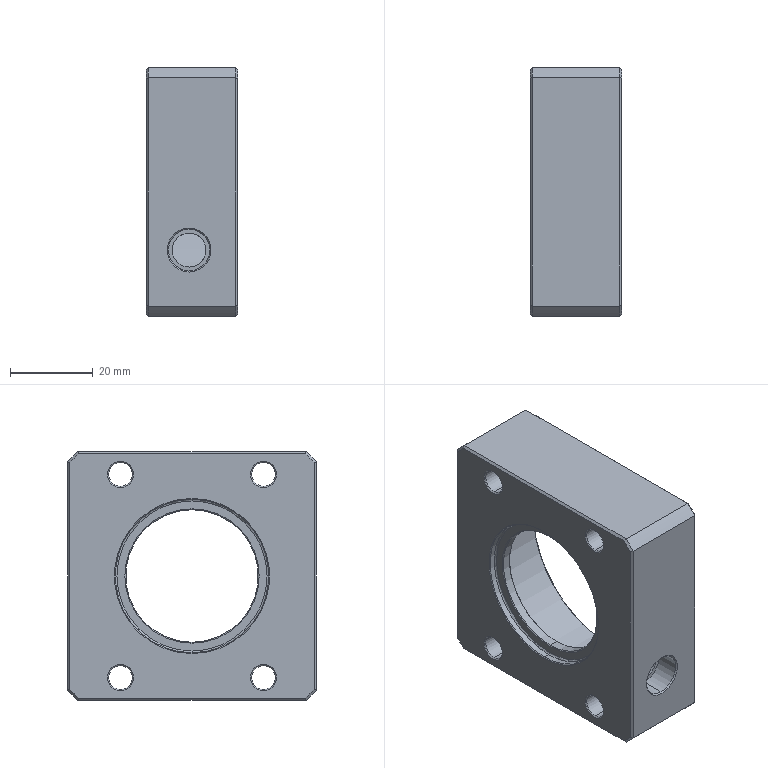Part | SolidWorks | features BaseBody 1 | 1 solid | 113 faces | box 22 x 60 x 60 mm | volume 35107 mm3 | cone 50 | cylinder 38 | plane 21 | torus 4 | commonest cylinder face diameters 3.3 x8 5.7 x8 9 x8 81.5 x4 8.2 x2 10 x2